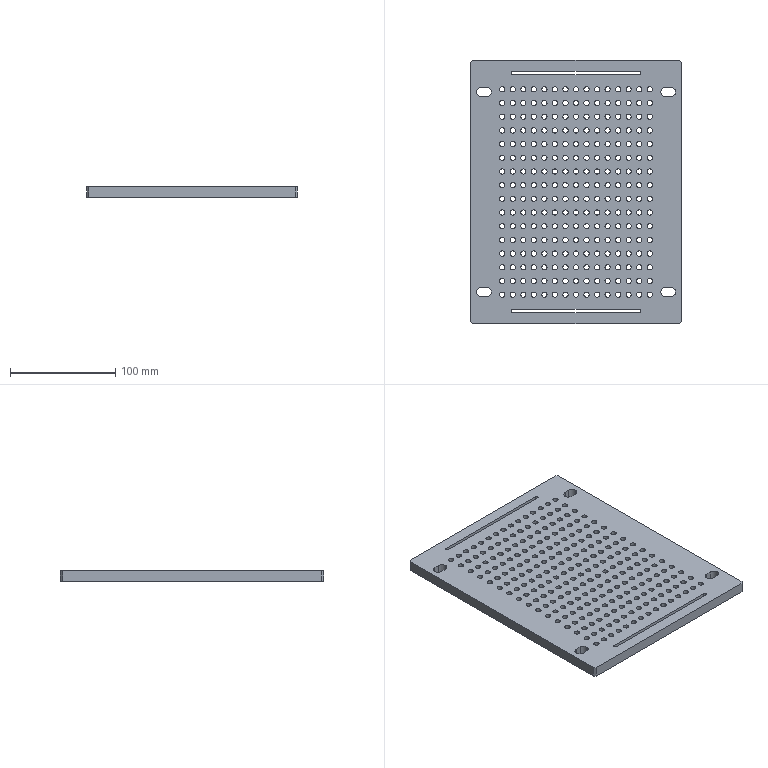Part | SolidWorks | features ICE 3, LPattern 3, Chamfer 1, Extrusion 1 | 1 solid | 520 faces | box 200 x 250 x 10 mm | volume 441110 mm3 | cylinder 498 | plane 22 | commonest cylinder face diameters 5 x480 9 x12 3 x6